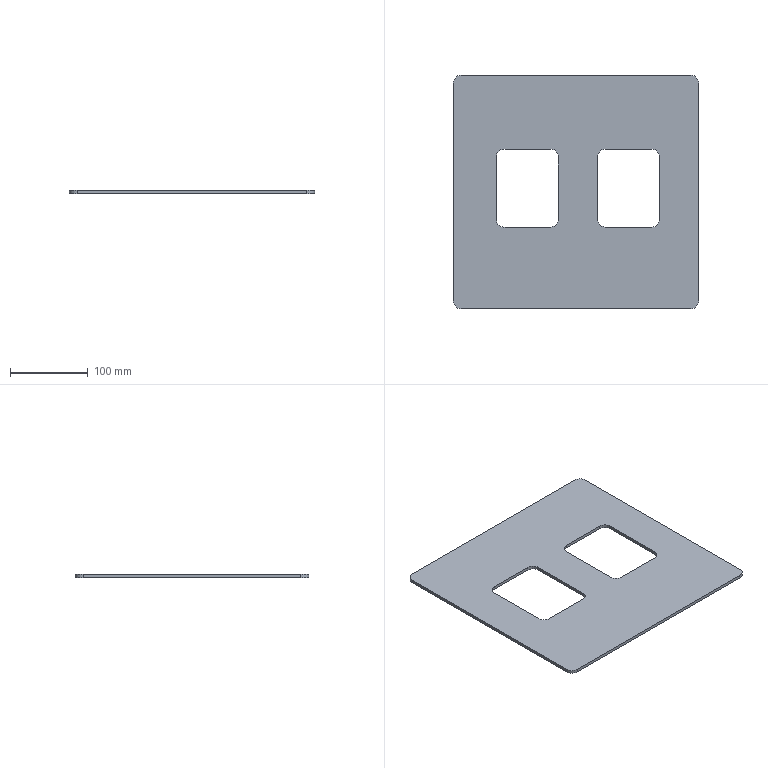Part | STEP file | transparent acrylic | 1 solid | 26 faces | box 315 x 300 x 4 mm | volume 314343 mm3 | plane 14 | cylinder 12 | commonest cylinder face diameters 20 x12